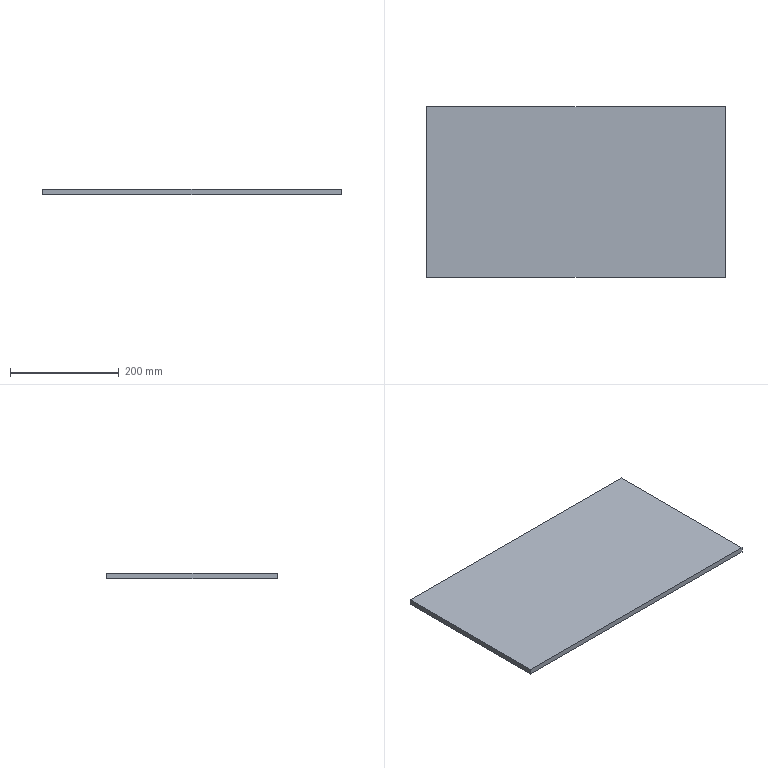Part | STEP file | 23.6 inch glass 001 | 1 solid | 6 faces | box 550 x 315 x 10 mm | volume 1732500 mm3 | plane 6
STEP:
#1=CARTESIAN_POINT('',(0.,0.,0.));
#2=DIRECTION('',(0.,0.,1.));
#3=DIRECTION('',(1.,0.,0.));
#4=AXIS2_PLACEMENT_3D('',#1,#2,#3);
#5=CARTESIAN_POINT('',(275.,-157.5,-5.));
#6=VERTEX_POINT('',#5);
#7=CARTESIAN_POINT('',(275.,157.5,-5.));
#8=VERTEX_POINT('',#7);
#9=CARTESIAN_POINT('',(275.,-157.5,-5.));
#10=DIRECTION('',(0.,1.,0.));
#11=VECTOR('',#10,1.);
#12=LINE('',#9,#11);
#13=CARTESIAN_POINT('',(275.,-157.5,5.));
#14=DIRECTION('',(-1.,0.,0.));
#15=DIRECTION('',(0.,0.,1.));
#16=AXIS2_PLACEMENT_3D('',#13,#14,#15);
#17=PLANE('',#16);
#18=CARTESIAN_POINT('',(-10.,0.));
#19=DIRECTION('',(0.,1.));
#20=VECTOR('',#19,1.);
#21=LINE('',#18,#20);
#22=(GEOMETRIC_REPRESENTATION_CONTEXT(2)PARAMETRIC_REPRESENTATION_CONTEXT()REPRESENTATION_CONTEXT('',''));
#23=DEFINITIONAL_REPRESENTATION('',(#21),#22);
#24=PCURVE('',#17,#23);
#25=CARTESIAN_POINT('',(0.,0.,-5.));
#26=DIRECTION('',(0.,0.,-1.));
#27=DIRECTION('',(-1.,0.,0.));
#28=AXIS2_PLACEMENT_3D('',#25,#26,#27);
#29=PLANE('',#28);
#30=CARTESIAN_POINT('',(-275.,-157.5));
#31=DIRECTION('',(0.,1.));
#32=VECTOR('',#31,1.);
#33=LINE('',#30,#32);
#34=(GEOMETRIC_REPRESENTATION_CONTEXT(2)PARAMETRIC_REPRESENTATION_CONTEXT()REPRESENTATION_CONTEXT('',''));
#35=DEFINITIONAL_REPRESENTATION('',(#33),#34);
#36=PCURVE('',#29,#35);
#37=SURFACE_CURVE('',#12,(#24,#36),.PCURVE_S1.);
#38=EDGE_CURVE('',#6,#8,#37,.T.);
#39=ORIENTED_EDGE('',*,*,#38,.T.);
#40=CARTESIAN_POINT('',(275.,157.5,5.));
#41=VERTEX_POINT('',#40);
#42=CARTESIAN_POINT('',(275.,157.5,5.));
#43=DIRECTION('',(0.,0.,-1.));
#44=VECTOR('',#43,1.);
#45=LINE('',#42,#44);
#46=CARTESIAN_POINT('',(0.,315.));
#47=DIRECTION('',(-1.,0.));
#48=VECTOR('',#47,1.);
#49=LINE('',#46,#48);
#50=(GEOMETRIC_REPRESENTATION_CONTEXT(2)PARAMETRIC_REPRESENTATION_CONTEXT()REPRESENTATION_CONTEXT('',''));
#51=DEFINITIONAL_REPRESENTATION('',(#49),#50);
#52=PCURVE('',#17,#51);
#53=CARTESIAN_POINT('',(-275.,157.5,5.));
#54=DIRECTION('',(0.,-1.,0.));
#55=DIRECTION('',(0.,0.,-1.));
#56=AXIS2_PLACEMENT_3D('',#53,#54,#55);
#57=PLANE('',#56);
#58=CARTESIAN_POINT('',(0.,550.));
#59=DIRECTION('',(1.,0.));
#60=VECTOR('',#59,1.);
#61=LINE('',#58,#60);
#62=(GEOMETRIC_REPRESENTATION_CONTEXT(2)PARAMETRIC_REPRESENTATION_CONTEXT()REPRESENTATION_CONTEXT('',''));
#63=DEFINITIONAL_REPRESENTATION('',(#61),#62);
#64=PCURVE('',#57,#63);
#65=SURFACE_CURVE('',#45,(#52,#64),.PCURVE_S1.);
#66=EDGE_CURVE('',#41,#8,#65,.T.);
#67=ORIENTED_EDGE('',*,*,#66,.F.);
#68=CARTESIAN_POINT('',(275.,-157.5,5.));
#69=VERTEX_POINT('',#68);
#70=CARTESIAN_POINT('',(275.,-157.5,5.));
#71=DIRECTION('',(0.,1.,0.));
#72=VECTOR('',#71,1.);
#73=LINE('',#70,#72);
#74=CARTESIAN_POINT('',(0.,0.));
#75=DIRECTION('',(0.,1.));
#76=VECTOR('',#75,1.);
#77=LINE('',#74,#76);
#78=(GEOMETRIC_REPRESENTATION_CONTEXT(2)PARAMETRIC_REPRESENTATION_CONTEXT()REPRESENTATION_CONTEXT('',''));
#79=DEFINITIONAL_REPRESENTATION('',(#77),#78);
#80=PCURVE('',#17,#79);
#81=CARTESIAN_POINT('',(0.,0.,5.));
#82=DIRECTION('',(0.,0.,-1.));
#83=DIRECTION('',(-1.,0.,0.));
#84=AXIS2_PLACEMENT_3D('',#81,#82,#83);
#85=PLANE('',#84);
#86=CARTESIAN_POINT('',(-275.,-157.5));
#87=DIRECTION('',(0.,1.));
#88=VECTOR('',#87,1.);
#89=LINE('',#86,#88);
#90=(GEOMETRIC_REPRESENTATION_CONTEXT(2)PARAMETRIC_REPRESENTATION_CONTEXT()REPRESENTATION_CONTEXT('',''));
#91=DEFINITIONAL_REPRESENTATION('',(#89),#90);
#92=PCURVE('',#85,#91);
#93=SURFACE_CURVE('',#73,(#80,#92),.PCURVE_S1.);
#94=EDGE_CURVE('',#69,#41,#93,.T.);
#95=ORIENTED_EDGE('',*,*,#94,.F.);
#96=CARTESIAN_POINT('',(275.,-157.5,5.));
#97=DIRECTION('',(0.,0.,-1.));
#98=VECTOR('',#97,1.);
#99=LINE('',#96,#98);
#100=CARTESIAN_POINT('',(0.,0.));
#101=DIRECTION('',(-1.,0.));
#102=VECTOR('',#101,1.);
#103=LINE('',#100,#102);
#104=(GEOMETRIC_REPRESENTATION_CONTEXT(2)PARAMETRIC_REPRESENTATION_CONTEXT()REPRESENTATION_CONTEXT('',''));
#105=DEFINITIONAL_REPRESENTATION('',(#103),#104);
#106=PCURVE('',#17,#105);
#107=CARTESIAN_POINT('',(-275.,-157.5,5.));
#108=DIRECTION('',(0.,1.,0.));
#109=DIRECTION('',(0.,0.,1.));
#110=AXIS2_PLACEMENT_3D('',#107,#108,#109);
#111=PLANE('',#110);
#112=CARTESIAN_POINT('',(0.,550.));
#113=DIRECTION('',(-1.,0.));
#114=VECTOR('',#113,1.);
#115=LINE('',#112,#114);
#116=(GEOMETRIC_REPRESENTATION_CONTEXT(2)PARAMETRIC_REPRESENTATION_CONTEXT()REPRESENTATION_CONTEXT('',''));
#117=DEFINITIONAL_REPRESENTATION('',(#115),#116);
#118=PCURVE('',#111,#117);
#119=SURFACE_CURVE('',#99,(#106,#118),.PCURVE_S1.);
#120=EDGE_CURVE('',#69,#6,#119,.T.);
#121=ORIENTED_EDGE('',*,*,#120,.T.);
#122=EDGE_LOOP('',(#39,#67,#95,#121));
#123=FACE_BOUND('',#122,.T.);
#124=ADVANCED_FACE('',(#123),#17,.F.);
#125=CARTESIAN_POINT('',(-275.,157.5,-5.));
#126=VERTEX_POINT('',#125);
#127=CARTESIAN_POINT('',(-275.,157.5,-5.));
#128=DIRECTION('',(-1.,0.,0.));
#129=VECTOR('',#128,1.);
#130=LINE('',#127,#129);
#131=CARTESIAN_POINT('',(10.,0.));
#132=DIRECTION('',(0.,-1.));
#133=VECTOR('',#132,1.);
#134=LINE('',#131,#133);
#135=(GEOMETRIC_REPRESENTATION_CONTEXT(2)PARAMETRIC_REPRESENTATION_CONTEXT()REPRESENTATION_CONTEXT('',''));
#136=DEFINITIONAL_REPRESENTATION('',(#134),#135);
#137=PCURVE('',#57,#136);
#138=CARTESIAN_POINT('',(275.,157.5));
#139=DIRECTION('',(1.,0.));
#140=VECTOR('',#139,1.);
#141=LINE('',#138,#140);
#142=(GEOMETRIC_REPRESENTATION_CONTEXT(2)PARAMETRIC_REPRESENTATION_CONTEXT()REPRESENTATION_CONTEXT('',''));
#143=DEFINITIONAL_REPRESENTATION('',(#141),#142);
#144=PCURVE('',#29,#143);
#145=SURFACE_CURVE('',#130,(#137,#144),.PCURVE_S1.);
#146=EDGE_CURVE('',#8,#126,#145,.T.);
#147=ORIENTED_EDGE('',*,*,#146,.T.);
#148=CARTESIAN_POINT('',(-275.,157.5,5.));
#149=VERTEX_POINT('',#148);
#150=CARTESIAN_POINT('',(-275.,157.5,5.));
#151=DIRECTION('',(0.,0.,-1.));
#152=VECTOR('',#151,1.);
#153=LINE('',#150,#152);
#154=CARTESIAN_POINT('',(0.,0.));
#155=DIRECTION('',(1.,0.));
#156=VECTOR('',#155,1.);
#157=LINE('',#154,#156);
#158=(GEOMETRIC_REPRESENTATION_CONTEXT(2)PARAMETRIC_REPRESENTATION_CONTEXT()REPRESENTATION_CONTEXT('',''));
#159=DEFINITIONAL_REPRESENTATION('',(#157),#158);
#160=PCURVE('',#57,#159);
#161=CARTESIAN_POINT('',(-275.,-157.5,5.));
#162=DIRECTION('',(1.,0.,0.));
#163=DIRECTION('',(0.,0.,-1.));
#164=AXIS2_PLACEMENT_3D('',#161,#162,#163);
#165=PLANE('',#164);
#166=CARTESIAN_POINT('',(0.,315.));
#167=DIRECTION('',(1.,0.));
#168=VECTOR('',#167,1.);
#169=LINE('',#166,#168);
#170=(GEOMETRIC_REPRESENTATION_CONTEXT(2)PARAMETRIC_REPRESENTATION_CONTEXT()REPRESENTATION_CONTEXT('',''));
#171=DEFINITIONAL_REPRESENTATION('',(#169),#170);
#172=PCURVE('',#165,#171);
#173=SURFACE_CURVE('',#153,(#160,#172),.PCURVE_S1.);
#174=EDGE_CURVE('',#149,#126,#173,.T.);
#175=ORIENTED_EDGE('',*,*,#174,.F.);
#176=CARTESIAN_POINT('',(-275.,157.5,5.));
#177=DIRECTION('',(-1.,0.,0.));
#178=VECTOR('',#177,1.);
#179=LINE('',#176,#178);
#180=CARTESIAN_POINT('',(0.,0.));
#181=DIRECTION('',(0.,-1.));
#182=VECTOR('',#181,1.);
#183=LINE('',#180,#182);
#184=(GEOMETRIC_REPRESENTATION_CONTEXT(2)PARAMETRIC_REPRESENTATION_CONTEXT()REPRESENTATION_CONTEXT('',''));
#185=DEFINITIONAL_REPRESENTATION('',(#183),#184);
#186=PCURVE('',#57,#185);
#187=CARTESIAN_POINT('',(275.,157.5));
#188=DIRECTION('',(1.,0.));
#189=VECTOR('',#188,1.);
#190=LINE('',#187,#189);
#191=(GEOMETRIC_REPRESENTATION_CONTEXT(2)PARAMETRIC_REPRESENTATION_CONTEXT()REPRESENTATION_CONTEXT('',''));
#192=DEFINITIONAL_REPRESENTATION('',(#190),#191);
#193=PCURVE('',#85,#192);
#194=SURFACE_CURVE('',#179,(#186,#193),.PCURVE_S1.);
#195=EDGE_CURVE('',#41,#149,#194,.T.);
#196=ORIENTED_EDGE('',*,*,#195,.F.);
#197=ORIENTED_EDGE('',*,*,#66,.T.);
#198=EDGE_LOOP('',(#147,#175,#196,#197));
#199=FACE_BOUND('',#198,.T.);
#200=ADVANCED_FACE('',(#199),#57,.F.);
#201=CARTESIAN_POINT('',(-275.,-157.5,-5.));
#202=VERTEX_POINT('',#201);
#203=CARTESIAN_POINT('',(-275.,-157.5,-5.));
#204=DIRECTION('',(0.,-1.,0.));
#205=VECTOR('',#204,1.);
#206=LINE('',#203,#205);
#207=CARTESIAN_POINT('',(10.,0.));
#208=DIRECTION('',(0.,-1.));
#209=VECTOR('',#208,1.);
#210=LINE('',#207,#209);
#211=(GEOMETRIC_REPRESENTATION_CONTEXT(2)PARAMETRIC_REPRESENTATION_CONTEXT()REPRESENTATION_CONTEXT('',''));
#212=DEFINITIONAL_REPRESENTATION('',(#210),#211);
#213=PCURVE('',#165,#212);
#214=CARTESIAN_POINT('',(275.,-157.5));
#215=DIRECTION('',(0.,-1.));
#216=VECTOR('',#215,1.);
#217=LINE('',#214,#216);
#218=(GEOMETRIC_REPRESENTATION_CONTEXT(2)PARAMETRIC_REPRESENTATION_CONTEXT()REPRESENTATION_CONTEXT('',''));
#219=DEFINITIONAL_REPRESENTATION('',(#217),#218);
#220=PCURVE('',#29,#219);
#221=SURFACE_CURVE('',#206,(#213,#220),.PCURVE_S1.);
#222=EDGE_CURVE('',#126,#202,#221,.T.);
#223=ORIENTED_EDGE('',*,*,#222,.T.);
#224=CARTESIAN_POINT('',(-275.,-157.5,5.));
#225=VERTEX_POINT('',#224);
#226=CARTESIAN_POINT('',(-275.,-157.5,5.));
#227=DIRECTION('',(0.,0.,-1.));
#228=VECTOR('',#227,1.);
#229=LINE('',#226,#228);
#230=CARTESIAN_POINT('',(0.,0.));
#231=DIRECTION('',(1.,0.));
#232=VECTOR('',#231,1.);
#233=LINE('',#230,#232);
#234=(GEOMETRIC_REPRESENTATION_CONTEXT(2)PARAMETRIC_REPRESENTATION_CONTEXT()REPRESENTATION_CONTEXT('',''));
#235=DEFINITIONAL_REPRESENTATION('',(#233),#234);
#236=PCURVE('',#165,#235);
#237=CARTESIAN_POINT('',(0.,0.));
#238=DIRECTION('',(-1.,0.));
#239=VECTOR('',#238,1.);
#240=LINE('',#237,#239);
#241=(GEOMETRIC_REPRESENTATION_CONTEXT(2)PARAMETRIC_REPRESENTATION_CONTEXT()REPRESENTATION_CONTEXT('',''));
#242=DEFINITIONAL_REPRESENTATION('',(#240),#241);
#243=PCURVE('',#111,#242);
#244=SURFACE_CURVE('',#229,(#236,#243),.PCURVE_S1.);
#245=EDGE_CURVE('',#225,#202,#244,.T.);
#246=ORIENTED_EDGE('',*,*,#245,.F.);
#247=CARTESIAN_POINT('',(-275.,-157.5,5.));
#248=DIRECTION('',(0.,-1.,0.));
#249=VECTOR('',#248,1.);
#250=LINE('',#247,#249);
#251=CARTESIAN_POINT('',(0.,0.));
#252=DIRECTION('',(0.,-1.));
#253=VECTOR('',#252,1.);
#254=LINE('',#251,#253);
#255=(GEOMETRIC_REPRESENTATION_CONTEXT(2)PARAMETRIC_REPRESENTATION_CONTEXT()REPRESENTATION_CONTEXT('',''));
#256=DEFINITIONAL_REPRESENTATION('',(#254),#255);
#257=PCURVE('',#165,#256);
#258=CARTESIAN_POINT('',(275.,-157.5));
#259=DIRECTION('',(0.,-1.));
#260=VECTOR('',#259,1.);
#261=LINE('',#258,#260);
#262=(GEOMETRIC_REPRESENTATION_CONTEXT(2)PARAMETRIC_REPRESENTATION_CONTEXT()REPRESENTATION_CONTEXT('',''));
#263=DEFINITIONAL_REPRESENTATION('',(#261),#262);
#264=PCURVE('',#85,#263);
#265=SURFACE_CURVE('',#250,(#257,#264),.PCURVE_S1.);
#266=EDGE_CURVE('',#149,#225,#265,.T.);
#267=ORIENTED_EDGE('',*,*,#266,.F.);
#268=ORIENTED_EDGE('',*,*,#174,.T.);
#269=EDGE_LOOP('',(#223,#246,#267,#268));
#270=FACE_BOUND('',#269,.T.);
#271=ADVANCED_FACE('',(#270),#165,.F.);
#272=CARTESIAN_POINT('',(-275.,-157.5,-5.));
#273=DIRECTION('',(1.,0.,0.));
#274=VECTOR('',#273,1.);
#275=LINE('',#272,#274);
#276=CARTESIAN_POINT('',(-10.,0.));
#277=DIRECTION('',(0.,1.));
#278=VECTOR('',#277,1.);
#279=LINE('',#276,#278);
#280=(GEOMETRIC_REPRESENTATION_CONTEXT(2)PARAMETRIC_REPRESENTATION_CONTEXT()REPRESENTATION_CONTEXT('',''));
#281=DEFINITIONAL_REPRESENTATION('',(#279),#280);
#282=PCURVE('',#111,#281);
#283=CARTESIAN_POINT('',(275.,-157.5));
#284=DIRECTION('',(-1.,0.));
#285=VECTOR('',#284,1.);
#286=LINE('',#283,#285);
#287=(GEOMETRIC_REPRESENTATION_CONTEXT(2)PARAMETRIC_REPRESENTATION_CONTEXT()REPRESENTATION_CONTEXT('',''));
#288=DEFINITIONAL_REPRESENTATION('',(#286),#287);
#289=PCURVE('',#29,#288);
#290=SURFACE_CURVE('',#275,(#282,#289),.PCURVE_S1.);
#291=EDGE_CURVE('',#202,#6,#290,.T.);
#292=ORIENTED_EDGE('',*,*,#291,.T.);
#293=ORIENTED_EDGE('',*,*,#120,.F.);
#294=CARTESIAN_POINT('',(-275.,-157.5,5.));
#295=DIRECTION('',(1.,0.,0.));
#296=VECTOR('',#295,1.);
#297=LINE('',#294,#296);
#298=CARTESIAN_POINT('',(0.,0.));
#299=DIRECTION('',(0.,1.));
#300=VECTOR('',#299,1.);
#301=LINE('',#298,#300);
#302=(GEOMETRIC_REPRESENTATION_CONTEXT(2)PARAMETRIC_REPRESENTATION_CONTEXT()REPRESENTATION_CONTEXT('',''));
#303=DEFINITIONAL_REPRESENTATION('',(#301),#302);
#304=PCURVE('',#111,#303);
#305=CARTESIAN_POINT('',(275.,-157.5));
#306=DIRECTION('',(-1.,0.));
#307=VECTOR('',#306,1.);
#308=LINE('',#305,#307);
#309=(GEOMETRIC_REPRESENTATION_CONTEXT(2)PARAMETRIC_REPRESENTATION_CONTEXT()REPRESENTATION_CONTEXT('',''));
#310=DEFINITIONAL_REPRESENTATION('',(#308),#309);
#311=PCURVE('',#85,#310);
#312=SURFACE_CURVE('',#297,(#304,#311),.PCURVE_S1.);
#313=EDGE_CURVE('',#225,#69,#312,.T.);
#314=ORIENTED_EDGE('',*,*,#313,.F.);
#315=ORIENTED_EDGE('',*,*,#245,.T.);
#316=EDGE_LOOP('',(#292,#293,#314,#315));
#317=FACE_BOUND('',#316,.T.);
#318=ADVANCED_FACE('',(#317),#111,.F.);
#319=ORIENTED_EDGE('',*,*,#94,.T.);
#320=ORIENTED_EDGE('',*,*,#195,.T.);
#321=ORIENTED_EDGE('',*,*,#266,.T.);
#322=ORIENTED_EDGE('',*,*,#313,.T.);
#323=EDGE_LOOP('',(#319,#320,#321,#322));
#324=FACE_BOUND('',#323,.T.);
#325=ADVANCED_FACE('',(#324),#85,.F.);
#326=ORIENTED_EDGE('',*,*,#38,.F.);
#327=ORIENTED_EDGE('',*,*,#291,.F.);
#328=ORIENTED_EDGE('',*,*,#222,.F.);
#329=ORIENTED_EDGE('',*,*,#146,.F.);
#330=EDGE_LOOP('',(#326,#327,#328,#329));
#331=FACE_BOUND('',#330,.T.);
#332=ADVANCED_FACE('',(#331),#29,.T.);
#333=CLOSED_SHELL('',(#124,#200,#271,#318,#325,#332));
#334=MANIFOLD_SOLID_BREP('',#333);
#335=(LENGTH_UNIT()NAMED_UNIT(*)SI_UNIT(.MILLI.,.METRE.));
#336=UNCERTAINTY_MEASURE_WITH_UNIT(LENGTH_MEASURE(0.0000001),#335,'','');
#337=(NAMED_UNIT(*)PLANE_ANGLE_UNIT()SI_UNIT($,.RADIAN.));
#338=(NAMED_UNIT(*)SI_UNIT($,.STERADIAN.)SOLID_ANGLE_UNIT());
#339=(GEOMETRIC_REPRESENTATION_CONTEXT(3)GLOBAL_UNCERTAINTY_ASSIGNED_CONTEXT((#336))GLOBAL_UNIT_ASSIGNED_CONTEXT((#335,#337,#338))REPRESENTATION_CONTEXT('',''));
#340=ADVANCED_BREP_SHAPE_REPRESENTATION('',(#4,#334),#339);